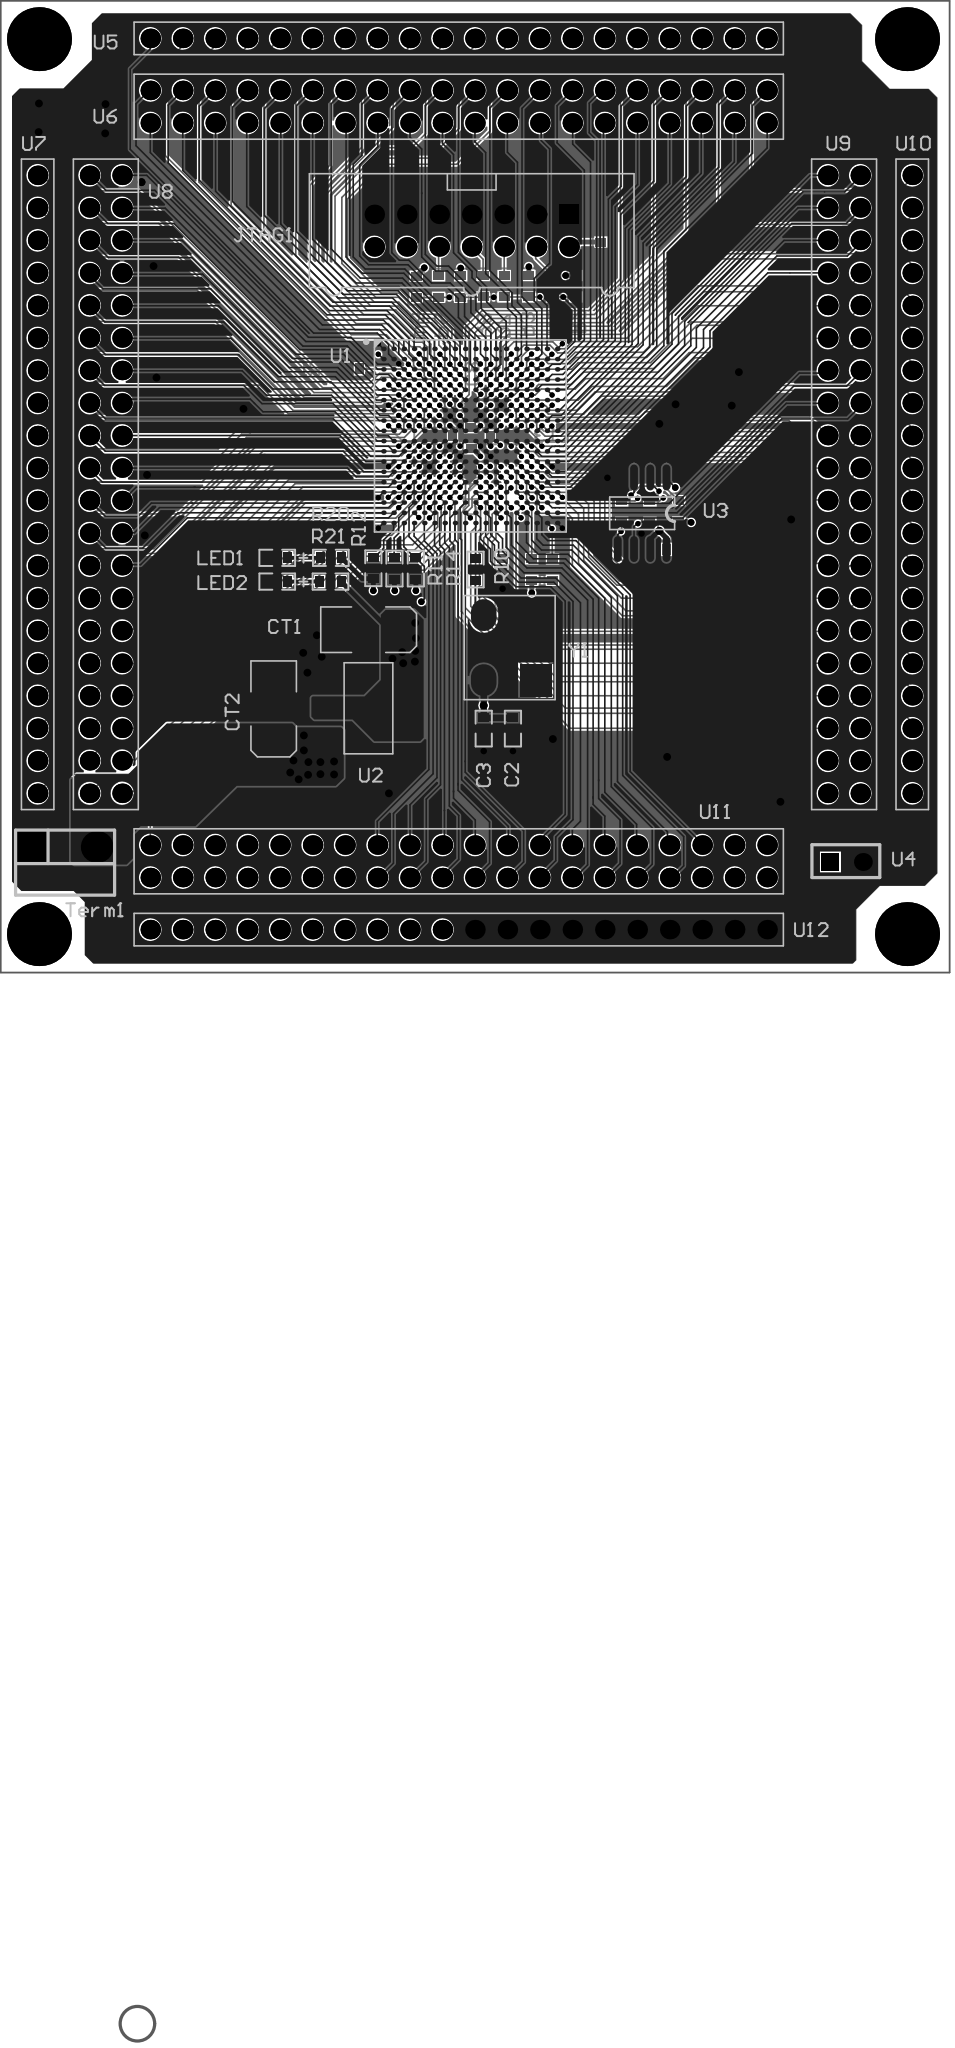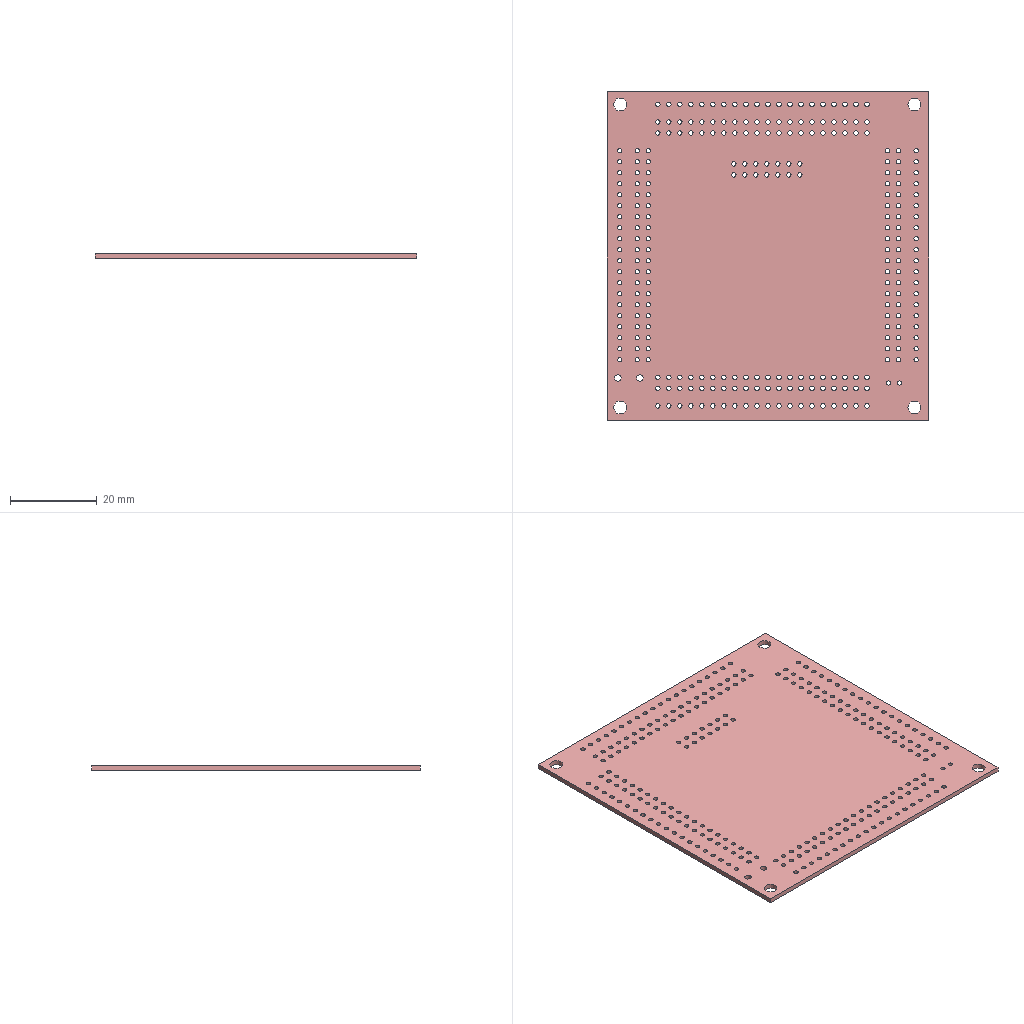Circuit board layout | Altium Designer | box 74.2 x 75.9 x 1.1 mm
Layer stack:
# Altium Designer layer stack of  (unit mm; dielectric type: 0 none, 1 core, 2 prepreg, 3 surface material)
index,name,kind,layer,copper_thickness_mm,dielectric_type,dielectric_thickness_mm,dielectric_material,dielectric_constant
0,Top Paste,other,,,,,,
1,Top Overlay,other,,,,,,
2,Top Solder,dielectric,,,3,0.0102,Solder Resist,3.5
3,Top Layer,copper,Top Layer,0.0356,,,,
4,Dielectric1,dielectric,,,1,0.32,FR-4,4.8
5,GND,copper,GND,0.0356,,,,
6,Dielectric2,dielectric,,,2,0.32,FR-4,4.8
7,POWER,copper,POWER,0.0356,,,,
8,Dielectric3,dielectric,,,1,0.32,FR-4,4.8
9,Bottom Layer,copper,Bottom Layer,0.0356,,,,
10,Bottom Solder,dielectric,,,3,0.0102,Solder Resist,3.5
11,Bottom Overlay,other,,,,,,
12,Bottom Paste,other,,,,,,
# drill layer pairs: low layer,high layer
drill_pair,Top Layer,Bottom Layer
Part placement:
Designator,Comment,Layer,Footprint,Center-X(mm),Center-Y(mm),Rotation
R15,4.7k,BottomLayer,0603,41.554,31.471,90
R18,22,BottomLayer,0603,39.268,31.471,90
C1,0.1u,BottomLayer,0603,46.965,57.887,270
R19,22,BottomLayer,0603,48.59,35.992,270
R9,51,BottomLayer,0603,34.265,53.569,90
R8,51,BottomLayer,0603,37.744,53.594,90
R5,10k,BottomLayer,0603,32.512,53.543,270
R4,10k,BottomLayer,0603,35.992,53.569,270
R3,10k,BottomLayer,0603,41.326,53.594,270
R2,10k,BottomLayer,0603,44.983,53.594,270
R17,22,BottomLayer,0603,50.8,35.992,270
R16,4.7k,BottomLayer,0603,53.061,36.017,270
R7,51,BottomLayer,0603,39.395,53.594,90
R6,51,BottomLayer,0603,43.18,53.594,90
R1,51,BottomLayer,0603,27.229,47.142,360
C4,0.1u,BottomLayer,0603,51.257,33.045,180
R13,4.7k,BottomLayer,0603,43.18,31.471,90
ZD1,T3V3S5,BottomLayer,0603,21.336,16.459,270
C7,0.1uF,BottomLayer,0603,34.519,41.91,360
C8,0.1uF,BottomLayer,0603,36.779,43.383,270
C13,0.1uF,BottomLayer,0603,39.141,41.885,180
C14,0.1uF,BottomLayer,0603,36.805,40.056,90
C2,0.1uF,TopLayer,0603,40.081,19.05,90
C3,0.1uF,TopLayer,0603,37.795,19.05,90
U6,TP20*2_2.54mm,TopLayer,TP20*2_2.54mm,35.839,67.615,0
U5,TP20_2.54mm,TopLayer,TP20_2.54mm,35.839,72.949,0
U8,TP20*2_2.54mm,TopLayer,TP20*2_2.54mm,8.23,38.125,270
U7,TP20_2.54mm,TopLayer,TP20_2.54mm,2.896,38.125,270
U9,TP20*2_2.54mm,TopLayer,TP20*2_2.54mm,65.989,38.125,270
U10,TP20_2.54mm,TopLayer,TP20_2.54mm,71.323,38.125,270
U11,TP20*2_2.54mm,TopLayer,TP20*2_2.54mm,35.839,8.687,0
U12,TP20_2.54mm,TopLayer,TP20_2.54mm,35.839,3.353,360
U2,LM1117-1.2V,TopLayer,SOT223,28.778,20.637,270
R14,4.7k,TopLayer,0603,32.487,31.547,90
R12,4.7k,TopLayer,0603,29.159,31.572,90
CT1,22u/10V,TopLayer,7227,28.791,26.772,360
CT2,22u/10V,TopLayer,7227,21.361,20.587,270
Y1,30MHz-3.3V,TopLayer,OSC-SO4,39.827,25.375,90
R11,4.7k,TopLayer,0603,30.81,31.547,90
R10,22,TopLayer,0603,37.16,31.471,90
U4,TP2,TopLayer,TP2,66.192,8.636,360
U3,M25P80,TopLayer,M25P16_SO-8,50.19,35.865,270
R20,2k,TopLayer,0603,25.832,32.385,360
R21,2k,TopLayer,0603,25.806,30.531,360
U1,XC6SLX9-CSG324,TopLayer,CSG324,36.747,41.903,0
JTAG1,JTAG,TopLayer,IDC14S,36.855,57.937,180
LED1,LED,TopLayer,DIODE_2,21.641,32.385,180
LED2,LED,TopLayer,DIODE_2,21.641,30.531,180
Term1,Phonix Connector 2p,TopLayer,PhonixCon2P,4.978,9.804,360
Pad and via stacks:
# Altium Designer via and pad stacks of  (unit mm). Each distinct definition once, with the count of objects using it.
# via: kind,start_layer,end_layer,hole_mm,diameter_mm,mode(0 simple;1 top-mid-bottom;2 full stack),diameter_per_layer,count,example_net
# pad: kind,layer,hole_mm,hole_type(0 round;1 square;2 slot),plating,top_size,top_shape(1 round;2 rect;3 octagon;9 rounded rect),mid_size,bottom_size,mode,footprint,size_per_layer,count,example
pad,Top Layer,0,0,plated,0.36x0.36,1,0.36x0.36,0.36x0.36,0,CSG324,,324,U1.A1
pad,Top Layer,0,0,plated,0.635x0.8128,2,0.635x0.8128,0.635x0.8128,0,DIODE_2,,4,LED1.A
pad,Top Layer,0,0,plated,1.905x2.54,2,1.905x2.54,1.905x2.54,0,7227,,4,CT1.2
pad,Top Layer,0,0,plated,0.635x0.8128,2,0.635x0.8128,0.635x0.8128,0,0603,,16,R14.2
pad,Top Layer,0,0,plated,1.499x2.007,2,1.499x2.007,1.499x2.007,0,SOT223,,3,U2.3
pad,Top Layer,0,0,plated,3.81x2.007,2,3.81x2.007,3.81x2.007,0,SOT223,,1,U2.2
pad,Top Layer,0,0,plated,2.032x0.6096,1,2.032x0.6096,2.032x0.6096,0,M25P16_SO-8,,8,U3.1
pad,Top Layer,0,0,plated,2.5x2.5,2,2.5x2.5,2.5x2.5,0,OSC-SO4,,1,Y1.1
pad,Top Layer,0,0,plated,2x2.5,1,2x2.5,2x2.5,0,OSC-SO4,,3,Y1.4
pad,Bottom Layer,0,0,plated,0.635x0.8128,2,0.635x0.8128,0.635x0.8128,0,0603,,44,C14.2
pad,Multi-Layer,1.016,0,plated,1.524x1.524,1,1.524x1.524,1.524x1.524,0,TP20*2_2.54mm,,160,U9.39
pad,Multi-Layer,1.016,0,plated,1.524x1.524,1,1.524x1.524,1.524x1.524,0,TP20_2.54mm,,80,U7.20
pad,Multi-Layer,1.524,0,plated,2.489x2.489,1,2.489x2.489,2.489x2.489,0,PhonixCon2P,,1,Term1.2
pad,Multi-Layer,1.524,0,plated,2.489x2.489,2,2.489x2.489,2.489x2.489,0,PhonixCon2P,,1,Term1.1
pad,Multi-Layer,0.9652,0,plated,1.397x1.397,2,1.397x1.397,1.397x1.397,0,TP2,,1,U4.1
pad,Multi-Layer,0.9652,0,plated,1.397x1.397,1,1.397x1.397,1.397x1.397,0,TP2,,1,U4.2
pad,Multi-Layer,1.016,0,plated,1.524x1.524,2,1.524x1.524,1.524x1.524,0,IDC14S,,1,JTAG1.1
pad,Multi-Layer,1.016,0,plated,1.524x1.524,1,1.524x1.524,1.524x1.524,0,IDC14S,,13,JTAG1.2
pad,Multi-Layer,3,0,plated,5x5,1,5x5,5x5,0,,,4,0
via,Top Layer,Bottom Layer,0.2032,0.4064,0,,221,+3.3V
via,Top Layer,Bottom Layer,0.3048,0.6096,0,,43,GND
via,Top Layer,Bottom Layer,0.2286,0.4318,0,,3,TMS
via,Top Layer,Bottom Layer,0.254,0.508,0,,16,+3.3V
Copper pours:
name,layer,net,type(0 solid;1 hatched;2 none)
TopLayer-No Net,Top Layer,GND,0
TopLayer-No Net,Top Layer,+3.3V,0
TopLayer-No Net,Top Layer,+1.2V,0
TopLayer-No Net,POWER,+3.3V,0
TopLayer-No Net,POWER,+1.2V,0
TopLayer-No Net,Bottom Layer,GND,0
TopLayer-No Net,GND,GND,0
Design rules, without the lines most boards share:
# Altium Designer design rules of  (exported by Altium Designer, unit mm)
# columns: name | kind | enabled | priority | scope1 | scope2 | descriptor | typed fields (field=value)
NetAntennae | 56 | enabled | 1 | All | All | Net Antennae (Tolerance=0mm) (All) |
SilkToSilkClearance | 55 | enabled | 1 | All | All | Silk to Silk (Clearance=0mm) (All),(All) |
SilkscreenOverComponentPads | 54 | enabled | 1 | IsPad | All | Silk To Solder Mask (Clearance=0mm) (IsPad),(All) |
MinimumSolderMaskSliver | 53 | enabled | 1 | All | All | Minimum Solder Mask Sliver (Gap=0.152mm) (All),(All) |
HoleToHoleClearance | 52 | enabled | 1 | All | All | Hole To Hole Clearance (Gap=0.152mm) (All),(All) | gap=0.1524
DiffPairsRouting | 51 | enabled | 1 | All | All | Differential Pairs Uncoupled Length using the Gap Constraints (Min=0.254mm) (Max=0.254mm) (Prefered=0.254mm)  and Width Constraints (Min=0.381mm) (Max=0.381mm) (Prefered=0.381mm) (All) |
HoleSize | 42 | enabled | 1 | All | All | Hole Size Constraint (Min=0.025mm) (Max=12.7mm) (All) |
Height | 50 | enabled | 1 | All | All | Height Constraint (Min=0mm) (Max=25.4mm) (Prefered=12.7mm) (All) | min_height=0 max_height=25.4
ComponentClearance | 24 | enabled | 1 | All | All | Component Clearance Constraint ( Horizontal Gap = 0.254mm, Vertical Gap = 0.254mm ) (All),(All)  | gap=0.254
Testpoint | 43 | enabled | 1 | (IsPad And (OnTopLayer Or OnBottomLayer)) | All | Fabrication Testpoint Style (Under Component=Yes) ((IsPad And (OnTopLayer Or OnBottomLayer))) |
TestPointUsage | 44 | enabled | 1 | All | All | Fabrication Testpoint Usage (Valid =One Required, Allow multiple per net=No) (All) |
SolderMaskExpansion | 13 | enabled | 1 | All | All | Solder Mask Expansion (Expansion =0.102mm) (All) | expansion=0.1016
PasteMaskExpansion | 14 | enabled | 1 | All | All | Paste Mask Expansion (Expansion =0mm) (All) | expansion=0
RoutingVias | 11 | enabled | 1 | All | All | Routing Via (MinHoleWidth=0.203mm) (MaxHoleWidth=0.508mm) (PreferredHoleWidth=0.254mm) (MinWidth=0.406mm) (MaxWidth=0.762mm) (PreferedWidth=0.508mm) (All) | via_min_hole=0.2032 via_max_hole=0.508 via_preferred_diameter=0.508 via_preferred_hole=0.254
RoutingCorners | 10 | enabled | 1 | All | All | Routing Corners (Style=45-Degree) (Min Setback=2.54mm) (Max Setback=2.54mm) (All) |
Width | 2 | enabled | 1 | All | All | Width Constraint (Min=0.127mm) (Max=0.508mm) (Preferred=0.127mm) (All) |
PolygonConnect | 20 | enabled | 2 | All | All | Polygon Connect Rule(Direct Connect )(Conductor Width=0.254mm) (Relief Angle=90 Angle) (Entries=4) (Air Gap Width=0.254mm) (All),(All) | connect_style(0=relief,1=direct,2=none)=1 relief_conductor_width=0.254 relief_entries=4
PlaneClearance | 12 | enabled | 1 | All | All | Power Plane Clearance (Clearance =0.508mm) (All) | clearance=0.508
PlaneConnect | 6 | enabled | 1 | All | All | Power Plane Connect Rule(Relief Connect )(Expansion=0.508mm) (Conductor Width=0.254mm) (Air Gap=0.254mm) (Entries=4) (All) | relief_conductor_width=0.254 relief_entries=4 relief_expansion=0.508
Clearance | 0 | enabled | 1 | All | All | Clearance Constraint (Gap=0.127mm) (All),(All) | gap=0.127
PolygonConnect_1 | 20 | enabled | 1 | All | isvia | Polygon Connect Rule(Direct Connect )(Conductor Width=0.254mm) (Relief Angle=90 Angle) (Entries=4) (Air Gap Width=0.254mm) (All),(isvia) | connect_style(0=relief,1=direct,2=none)=1 relief_conductor_width=0.254 relief_entries=4